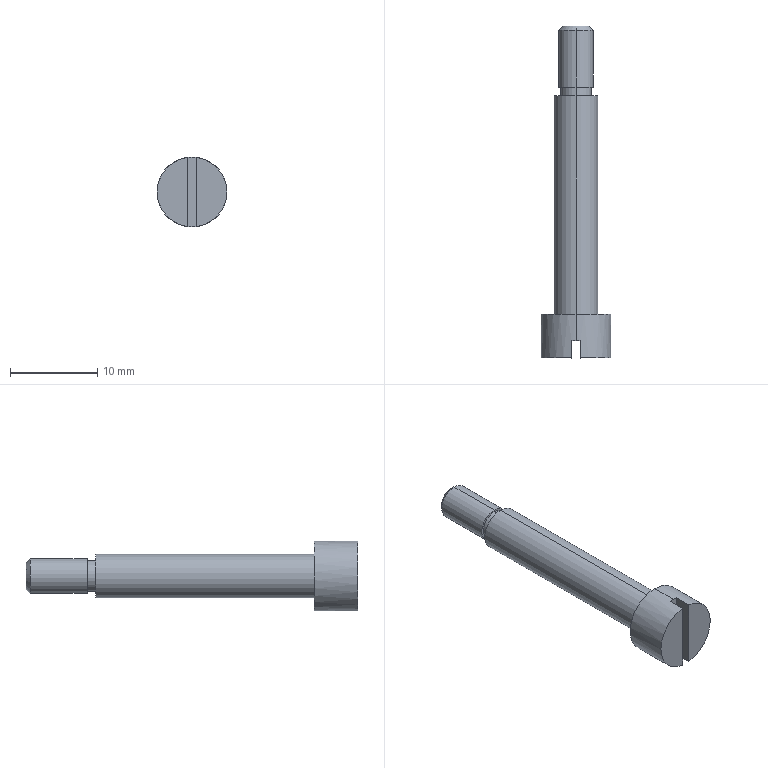Part | STEP file | 04-15 guide screw | 1 solid | 19 faces | box 8 x 38 x 8 mm | volume 822.389 mm3 | plane 9 | cylinder 8 | cone 2 | commonest cylinder face diameters 3.5 x2 4 x2 5 x2 8 x2
STEP:
#1=CARTESIAN_POINT('',(0.,7.,1.5));
#2=VERTEX_POINT('',#1);
#3=CARTESIAN_POINT('',(0.,7.,-1.5));
#4=VERTEX_POINT('',#3);
#5=CARTESIAN_POINT('',(0.,7.,0.));
#6=DIRECTION('',(0.,1.,0.));
#7=DIRECTION('',(0.,0.,1.));
#8=AXIS2_PLACEMENT_3D('',#5,#6,#7);
#9=CIRCLE('',#8,1.5);
#10=EDGE_CURVE('',#2,#4,#9,.T.);
#11=ORIENTED_EDGE('',*,*,#10,.F.);
#12=CARTESIAN_POINT('',(0.,6.5,2.));
#13=VERTEX_POINT('',#12);
#14=CARTESIAN_POINT('',(0.,7.,1.5));
#15=DIRECTION('',(0.,-0.7071,0.7071));
#16=VECTOR('',#15,1000.);
#17=LINE('',#14,#16);
#18=EDGE_CURVE('',#2,#13,#17,.T.);
#19=ORIENTED_EDGE('',*,*,#18,.T.);
#20=CARTESIAN_POINT('',(0.,6.5,-2.));
#21=VERTEX_POINT('',#20);
#22=CARTESIAN_POINT('',(0.,6.5,0.));
#23=DIRECTION('',(0.,-1.,0.));
#24=DIRECTION('',(0.,0.,1.));
#25=AXIS2_PLACEMENT_3D('',#22,#23,#24);
#26=CIRCLE('',#25,2.);
#27=EDGE_CURVE('',#21,#13,#26,.T.);
#28=ORIENTED_EDGE('',*,*,#27,.F.);
#29=CARTESIAN_POINT('',(0.,7.,-1.5));
#30=DIRECTION('',(0.,-0.7071,-0.7071));
#31=VECTOR('',#30,1000.);
#32=LINE('',#29,#31);
#33=EDGE_CURVE('',#4,#21,#32,.T.);
#34=ORIENTED_EDGE('',*,*,#33,.F.);
#35=EDGE_LOOP('',(#11,#19,#28,#34));
#36=FACE_OUTER_BOUND('',#35,.T.);
#37=CARTESIAN_POINT('',(0.,7.,0.));
#38=DIRECTION('',(0.,-1.,0.));
#39=DIRECTION('',(0.,0.,-1.));
#40=AXIS2_PLACEMENT_3D('',#37,#38,#39);
#41=CONICAL_SURFACE('',#40,1.5,0.7854);
#42=ADVANCED_FACE('',(#36),#41,.T.);
#43=CARTESIAN_POINT('',(0.,-29.,-4.));
#44=VERTEX_POINT('',#43);
#45=CARTESIAN_POINT('',(0.5,-29.,-3.969));
#46=VERTEX_POINT('',#45);
#47=CARTESIAN_POINT('',(0.,-29.,0.));
#48=DIRECTION('',(0.,-1.,0.));
#49=DIRECTION('',(0.,0.,-1.));
#50=AXIS2_PLACEMENT_3D('',#47,#48,#49);
#51=CIRCLE('',#50,4.);
#52=EDGE_CURVE('',#44,#46,#51,.T.);
#53=ORIENTED_EDGE('',*,*,#52,.F.);
#54=CARTESIAN_POINT('',(0.,-26.,-4.));
#55=VERTEX_POINT('',#54);
#56=CARTESIAN_POINT('',(0.,-31.,-4.));
#57=DIRECTION('',(0.,1.,0.));
#58=VECTOR('',#57,1000.);
#59=LINE('',#56,#58);
#60=EDGE_CURVE('',#44,#55,#59,.T.);
#61=ORIENTED_EDGE('',*,*,#60,.T.);
#62=CARTESIAN_POINT('',(0.,-26.,4.));
#63=VERTEX_POINT('',#62);
#64=CARTESIAN_POINT('',(0.,-26.,0.));
#65=DIRECTION('',(0.,-1.,0.));
#66=DIRECTION('',(0.,0.,-1.));
#67=AXIS2_PLACEMENT_3D('',#64,#65,#66);
#68=CIRCLE('',#67,4.);
#69=EDGE_CURVE('',#55,#63,#68,.T.);
#70=ORIENTED_EDGE('',*,*,#69,.T.);
#71=CARTESIAN_POINT('',(0.,-29.,4.));
#72=VERTEX_POINT('',#71);
#73=CARTESIAN_POINT('',(0.,-31.,4.));
#74=DIRECTION('',(0.,1.,0.));
#75=VECTOR('',#74,1000.);
#76=LINE('',#73,#75);
#77=EDGE_CURVE('',#72,#63,#76,.T.);
#78=ORIENTED_EDGE('',*,*,#77,.F.);
#79=CARTESIAN_POINT('',(0.5,-29.,3.969));
#80=VERTEX_POINT('',#79);
#81=CARTESIAN_POINT('',(0.,-29.,0.));
#82=DIRECTION('',(0.,-1.,0.));
#83=DIRECTION('',(0.,0.,-1.));
#84=AXIS2_PLACEMENT_3D('',#81,#82,#83);
#85=CIRCLE('',#84,4.);
#86=EDGE_CURVE('',#80,#72,#85,.T.);
#87=ORIENTED_EDGE('',*,*,#86,.F.);
#88=CARTESIAN_POINT('',(0.5,-31.,3.969));
#89=VERTEX_POINT('',#88);
#90=CARTESIAN_POINT('',(0.5,-31.,3.969));
#91=DIRECTION('',(0.,-1.,0.));
#92=VECTOR('',#91,1000.);
#93=LINE('',#90,#92);
#94=EDGE_CURVE('',#80,#89,#93,.T.);
#95=ORIENTED_EDGE('',*,*,#94,.T.);
#96=CARTESIAN_POINT('',(0.5,-31.,-3.969));
#97=VERTEX_POINT('',#96);
#98=CARTESIAN_POINT('',(0.,-31.,0.));
#99=DIRECTION('',(0.,-1.,0.));
#100=DIRECTION('',(0.,0.,-1.));
#101=AXIS2_PLACEMENT_3D('',#98,#99,#100);
#102=CIRCLE('',#101,4.);
#103=EDGE_CURVE('',#97,#89,#102,.T.);
#104=ORIENTED_EDGE('',*,*,#103,.F.);
#105=CARTESIAN_POINT('',(0.5,-31.,-3.969));
#106=DIRECTION('',(0.,1.,0.));
#107=VECTOR('',#106,1000.);
#108=LINE('',#105,#107);
#109=EDGE_CURVE('',#97,#46,#108,.T.);
#110=ORIENTED_EDGE('',*,*,#109,.T.);
#111=EDGE_LOOP('',(#53,#61,#70,#78,#87,#95,#104,#110));
#112=FACE_OUTER_BOUND('',#111,.T.);
#113=CARTESIAN_POINT('',(0.,-31.,0.));
#114=DIRECTION('',(0.,1.,0.));
#115=DIRECTION('',(0.,0.,1.));
#116=AXIS2_PLACEMENT_3D('',#113,#114,#115);
#117=CYLINDRICAL_SURFACE('',#116,4.);
#118=ADVANCED_FACE('',(#112),#117,.T.);
#119=CARTESIAN_POINT('',(0.,-26.,-2.5));
#120=VERTEX_POINT('',#119);
#121=CARTESIAN_POINT('',(0.,-26.,2.5));
#122=VERTEX_POINT('',#121);
#123=CARTESIAN_POINT('',(0.,-26.,0.));
#124=DIRECTION('',(0.,-1.,0.));
#125=DIRECTION('',(0.,0.,-1.));
#126=AXIS2_PLACEMENT_3D('',#123,#124,#125);
#127=CIRCLE('',#126,2.5);
#128=EDGE_CURVE('',#120,#122,#127,.T.);
#129=ORIENTED_EDGE('',*,*,#128,.F.);
#130=CARTESIAN_POINT('',(0.,-1.,-2.5));
#131=VERTEX_POINT('',#130);
#132=CARTESIAN_POINT('',(0.,-26.,-2.5));
#133=DIRECTION('',(0.,1.,0.));
#134=VECTOR('',#133,1000.);
#135=LINE('',#132,#134);
#136=EDGE_CURVE('',#120,#131,#135,.T.);
#137=ORIENTED_EDGE('',*,*,#136,.T.);
#138=CARTESIAN_POINT('',(0.,-1.,2.5));
#139=VERTEX_POINT('',#138);
#140=CARTESIAN_POINT('',(0.,-1.,0.));
#141=DIRECTION('',(0.,-1.,0.));
#142=DIRECTION('',(0.,0.,-1.));
#143=AXIS2_PLACEMENT_3D('',#140,#141,#142);
#144=CIRCLE('',#143,2.5);
#145=EDGE_CURVE('',#131,#139,#144,.T.);
#146=ORIENTED_EDGE('',*,*,#145,.T.);
#147=CARTESIAN_POINT('',(0.,-26.,2.5));
#148=DIRECTION('',(0.,1.,0.));
#149=VECTOR('',#148,1000.);
#150=LINE('',#147,#149);
#151=EDGE_CURVE('',#122,#139,#150,.T.);
#152=ORIENTED_EDGE('',*,*,#151,.F.);
#153=EDGE_LOOP('',(#129,#137,#146,#152));
#154=FACE_OUTER_BOUND('',#153,.T.);
#155=CARTESIAN_POINT('',(0.,-26.,0.));
#156=DIRECTION('',(0.,1.,0.));
#157=DIRECTION('',(0.,0.,1.));
#158=AXIS2_PLACEMENT_3D('',#155,#156,#157);
#159=CYLINDRICAL_SURFACE('',#158,2.5);
#160=ADVANCED_FACE('',(#154),#159,.T.);
#161=CARTESIAN_POINT('',(0.,-1.,-1.75));
#162=VERTEX_POINT('',#161);
#163=CARTESIAN_POINT('',(0.,-1.,1.75));
#164=VERTEX_POINT('',#163);
#165=CARTESIAN_POINT('',(0.,-1.,0.));
#166=DIRECTION('',(0.,-1.,0.));
#167=DIRECTION('',(0.,0.,-1.));
#168=AXIS2_PLACEMENT_3D('',#165,#166,#167);
#169=CIRCLE('',#168,1.75);
#170=EDGE_CURVE('',#162,#164,#169,.T.);
#171=ORIENTED_EDGE('',*,*,#170,.F.);
#172=CARTESIAN_POINT('',(0.,0.,-1.75));
#173=VERTEX_POINT('',#172);
#174=CARTESIAN_POINT('',(0.,-1.,-1.75));
#175=DIRECTION('',(0.,1.,0.));
#176=VECTOR('',#175,1000.);
#177=LINE('',#174,#176);
#178=EDGE_CURVE('',#162,#173,#177,.T.);
#179=ORIENTED_EDGE('',*,*,#178,.T.);
#180=CARTESIAN_POINT('',(0.,0.,1.75));
#181=VERTEX_POINT('',#180);
#182=CARTESIAN_POINT('',(0.,0.,0.));
#183=DIRECTION('',(0.,-1.,0.));
#184=DIRECTION('',(0.,0.,1.));
#185=AXIS2_PLACEMENT_3D('',#182,#183,#184);
#186=CIRCLE('',#185,1.75);
#187=EDGE_CURVE('',#173,#181,#186,.T.);
#188=ORIENTED_EDGE('',*,*,#187,.T.);
#189=CARTESIAN_POINT('',(0.,-1.,1.75));
#190=DIRECTION('',(0.,1.,0.));
#191=VECTOR('',#190,1000.);
#192=LINE('',#189,#191);
#193=EDGE_CURVE('',#164,#181,#192,.T.);
#194=ORIENTED_EDGE('',*,*,#193,.F.);
#195=EDGE_LOOP('',(#171,#179,#188,#194));
#196=FACE_OUTER_BOUND('',#195,.T.);
#197=CARTESIAN_POINT('',(0.,-1.,0.));
#198=DIRECTION('',(0.,1.,0.));
#199=DIRECTION('',(0.,0.,1.));
#200=AXIS2_PLACEMENT_3D('',#197,#198,#199);
#201=CYLINDRICAL_SURFACE('',#200,1.75);
#202=ADVANCED_FACE('',(#196),#201,.T.);
#203=ORIENTED_EDGE('',*,*,#27,.T.);
#204=CARTESIAN_POINT('',(0.,0.,2.));
#205=VERTEX_POINT('',#204);
#206=CARTESIAN_POINT('',(0.,7.,2.));
#207=DIRECTION('',(0.,-1.,0.));
#208=VECTOR('',#207,1000.);
#209=LINE('',#206,#208);
#210=EDGE_CURVE('',#13,#205,#209,.T.);
#211=ORIENTED_EDGE('',*,*,#210,.T.);
#212=CARTESIAN_POINT('',(0.,0.,-2.));
#213=VERTEX_POINT('',#212);
#214=CARTESIAN_POINT('',(0.,0.,0.));
#215=DIRECTION('',(0.,1.,0.));
#216=DIRECTION('',(0.,0.,1.));
#217=AXIS2_PLACEMENT_3D('',#214,#215,#216);
#218=CIRCLE('',#217,2.);
#219=EDGE_CURVE('',#205,#213,#218,.T.);
#220=ORIENTED_EDGE('',*,*,#219,.T.);
#221=CARTESIAN_POINT('',(0.,7.,-2.));
#222=DIRECTION('',(0.,-1.,0.));
#223=VECTOR('',#222,1000.);
#224=LINE('',#221,#223);
#225=EDGE_CURVE('',#21,#213,#224,.T.);
#226=ORIENTED_EDGE('',*,*,#225,.F.);
#227=EDGE_LOOP('',(#203,#211,#220,#226));
#228=FACE_OUTER_BOUND('',#227,.T.);
#229=CARTESIAN_POINT('',(0.,7.,0.));
#230=DIRECTION('',(0.,-1.,0.));
#231=DIRECTION('',(0.,0.,-1.));
#232=AXIS2_PLACEMENT_3D('',#229,#230,#231);
#233=CYLINDRICAL_SURFACE('',#232,2.);
#234=ADVANCED_FACE('',(#228),#233,.T.);
#235=CARTESIAN_POINT('',(0.5,-31.,0.));
#236=DIRECTION('',(0.,0.,1.));
#237=VECTOR('',#236,1000.);
#238=LINE('',#235,#237);
#239=EDGE_CURVE('',#97,#89,#238,.T.);
#240=ORIENTED_EDGE('',*,*,#239,.F.);
#241=ORIENTED_EDGE('',*,*,#103,.T.);
#242=EDGE_LOOP('',(#240,#241));
#243=FACE_OUTER_BOUND('',#242,.T.);
#244=CARTESIAN_POINT('',(0.,-31.,0.));
#245=DIRECTION('',(0.,-1.,0.));
#246=DIRECTION('',(0.,0.,-1.));
#247=AXIS2_PLACEMENT_3D('',#244,#245,#246);
#248=PLANE('',#247);
#249=ADVANCED_FACE('',(#243),#248,.T.);
#250=CARTESIAN_POINT('',(0.,0.,0.));
#251=DIRECTION('',(0.,1.,0.));
#252=DIRECTION('',(0.,0.,1.));
#253=AXIS2_PLACEMENT_3D('',#250,#251,#252);
#254=CIRCLE('',#253,2.);
#255=EDGE_CURVE('',#213,#205,#254,.T.);
#256=ORIENTED_EDGE('',*,*,#255,.F.);
#257=ORIENTED_EDGE('',*,*,#219,.F.);
#258=EDGE_LOOP('',(#256,#257));
#259=FACE_OUTER_BOUND('',#258,.T.);
#260=CARTESIAN_POINT('',(0.,0.,0.));
#261=DIRECTION('',(0.,-1.,0.));
#262=DIRECTION('',(0.,0.,1.));
#263=AXIS2_PLACEMENT_3D('',#260,#261,#262);
#264=CIRCLE('',#263,1.75);
#265=EDGE_CURVE('',#181,#173,#264,.T.);
#266=ORIENTED_EDGE('',*,*,#265,.F.);
#267=ORIENTED_EDGE('',*,*,#187,.F.);
#268=EDGE_LOOP('',(#266,#267));
#269=FACE_BOUND('',#268,.T.);
#270=CARTESIAN_POINT('',(0.,0.,0.));
#271=DIRECTION('',(0.,1.,0.));
#272=DIRECTION('',(0.,0.,1.));
#273=AXIS2_PLACEMENT_3D('',#270,#271,#272);
#274=PLANE('',#273);
#275=ADVANCED_FACE('',(#259,#269),#274,.F.);
#276=ORIENTED_EDGE('',*,*,#210,.F.);
#277=CARTESIAN_POINT('',(0.,6.5,0.));
#278=DIRECTION('',(0.,-1.,0.));
#279=DIRECTION('',(0.,0.,1.));
#280=AXIS2_PLACEMENT_3D('',#277,#278,#279);
#281=CIRCLE('',#280,2.);
#282=EDGE_CURVE('',#13,#21,#281,.T.);
#283=ORIENTED_EDGE('',*,*,#282,.T.);
#284=ORIENTED_EDGE('',*,*,#225,.T.);
#285=ORIENTED_EDGE('',*,*,#255,.T.);
#286=EDGE_LOOP('',(#276,#283,#284,#285));
#287=FACE_OUTER_BOUND('',#286,.T.);
#288=CARTESIAN_POINT('',(0.,7.,0.));
#289=DIRECTION('',(0.,-1.,0.));
#290=DIRECTION('',(0.,0.,-1.));
#291=AXIS2_PLACEMENT_3D('',#288,#289,#290);
#292=CYLINDRICAL_SURFACE('',#291,2.);
#293=ADVANCED_FACE('',(#287),#292,.T.);
#294=CARTESIAN_POINT('',(0.,7.,0.));
#295=DIRECTION('',(0.,1.,0.));
#296=DIRECTION('',(0.,0.,1.));
#297=AXIS2_PLACEMENT_3D('',#294,#295,#296);
#298=CIRCLE('',#297,1.5);
#299=EDGE_CURVE('',#4,#2,#298,.T.);
#300=ORIENTED_EDGE('',*,*,#299,.T.);
#301=ORIENTED_EDGE('',*,*,#10,.T.);
#302=EDGE_LOOP('',(#300,#301));
#303=FACE_OUTER_BOUND('',#302,.T.);
#304=CARTESIAN_POINT('',(0.,7.,0.));
#305=DIRECTION('',(0.,1.,0.));
#306=DIRECTION('',(0.,0.,1.));
#307=AXIS2_PLACEMENT_3D('',#304,#305,#306);
#308=PLANE('',#307);
#309=ADVANCED_FACE('',(#303),#308,.T.);
#310=ORIENTED_EDGE('',*,*,#178,.F.);
#311=CARTESIAN_POINT('',(0.,-1.,0.));
#312=DIRECTION('',(0.,-1.,0.));
#313=DIRECTION('',(0.,0.,-1.));
#314=AXIS2_PLACEMENT_3D('',#311,#312,#313);
#315=CIRCLE('',#314,1.75);
#316=EDGE_CURVE('',#164,#162,#315,.T.);
#317=ORIENTED_EDGE('',*,*,#316,.F.);
#318=ORIENTED_EDGE('',*,*,#193,.T.);
#319=ORIENTED_EDGE('',*,*,#265,.T.);
#320=EDGE_LOOP('',(#310,#317,#318,#319));
#321=FACE_OUTER_BOUND('',#320,.T.);
#322=CARTESIAN_POINT('',(0.,-1.,0.));
#323=DIRECTION('',(0.,1.,0.));
#324=DIRECTION('',(0.,0.,1.));
#325=AXIS2_PLACEMENT_3D('',#322,#323,#324);
#326=CYLINDRICAL_SURFACE('',#325,1.75);
#327=ADVANCED_FACE('',(#321),#326,.T.);
#328=CARTESIAN_POINT('',(0.,-1.,0.));
#329=DIRECTION('',(0.,-1.,0.));
#330=DIRECTION('',(0.,0.,-1.));
#331=AXIS2_PLACEMENT_3D('',#328,#329,#330);
#332=CIRCLE('',#331,2.5);
#333=EDGE_CURVE('',#139,#131,#332,.T.);
#334=ORIENTED_EDGE('',*,*,#333,.F.);
#335=ORIENTED_EDGE('',*,*,#145,.F.);
#336=EDGE_LOOP('',(#334,#335));
#337=FACE_OUTER_BOUND('',#336,.T.);
#338=ORIENTED_EDGE('',*,*,#316,.T.);
#339=ORIENTED_EDGE('',*,*,#170,.T.);
#340=EDGE_LOOP('',(#338,#339));
#341=FACE_BOUND('',#340,.T.);
#342=CARTESIAN_POINT('',(0.,-1.,0.));
#343=DIRECTION('',(0.,-1.,0.));
#344=DIRECTION('',(0.,0.,-1.));
#345=AXIS2_PLACEMENT_3D('',#342,#343,#344);
#346=PLANE('',#345);
#347=ADVANCED_FACE('',(#337,#341),#346,.F.);
#348=ORIENTED_EDGE('',*,*,#136,.F.);
#349=CARTESIAN_POINT('',(0.,-26.,0.));
#350=DIRECTION('',(0.,-1.,0.));
#351=DIRECTION('',(0.,0.,-1.));
#352=AXIS2_PLACEMENT_3D('',#349,#350,#351);
#353=CIRCLE('',#352,2.5);
#354=EDGE_CURVE('',#122,#120,#353,.T.);
#355=ORIENTED_EDGE('',*,*,#354,.F.);
#356=ORIENTED_EDGE('',*,*,#151,.T.);
#357=ORIENTED_EDGE('',*,*,#333,.T.);
#358=EDGE_LOOP('',(#348,#355,#356,#357));
#359=FACE_OUTER_BOUND('',#358,.T.);
#360=CARTESIAN_POINT('',(0.,-26.,0.));
#361=DIRECTION('',(0.,1.,0.));
#362=DIRECTION('',(0.,0.,1.));
#363=AXIS2_PLACEMENT_3D('',#360,#361,#362);
#364=CYLINDRICAL_SURFACE('',#363,2.5);
#365=ADVANCED_FACE('',(#359),#364,.T.);
#366=CARTESIAN_POINT('',(0.,-26.,0.));
#367=DIRECTION('',(0.,-1.,0.));
#368=DIRECTION('',(0.,0.,-1.));
#369=AXIS2_PLACEMENT_3D('',#366,#367,#368);
#370=CIRCLE('',#369,4.);
#371=EDGE_CURVE('',#63,#55,#370,.T.);
#372=ORIENTED_EDGE('',*,*,#371,.F.);
#373=ORIENTED_EDGE('',*,*,#69,.F.);
#374=EDGE_LOOP('',(#372,#373));
#375=FACE_OUTER_BOUND('',#374,.T.);
#376=ORIENTED_EDGE('',*,*,#354,.T.);
#377=ORIENTED_EDGE('',*,*,#128,.T.);
#378=EDGE_LOOP('',(#376,#377));
#379=FACE_BOUND('',#378,.T.);
#380=CARTESIAN_POINT('',(0.,-26.,0.));
#381=DIRECTION('',(0.,-1.,0.));
#382=DIRECTION('',(0.,0.,-1.));
#383=AXIS2_PLACEMENT_3D('',#380,#381,#382);
#384=PLANE('',#383);
#385=ADVANCED_FACE('',(#375,#379),#384,.F.);
#386=ORIENTED_EDGE('',*,*,#60,.F.);
#387=CARTESIAN_POINT('',(-0.5,-29.,-3.969));
#388=VERTEX_POINT('',#387);
#389=CARTESIAN_POINT('',(0.,-29.,0.));
#390=DIRECTION('',(0.,-1.,0.));
#391=DIRECTION('',(0.,0.,-1.));
#392=AXIS2_PLACEMENT_3D('',#389,#390,#391);
#393=CIRCLE('',#392,4.);
#394=EDGE_CURVE('',#388,#44,#393,.T.);
#395=ORIENTED_EDGE('',*,*,#394,.F.);
#396=CARTESIAN_POINT('',(-0.5,-31.,-3.969));
#397=VERTEX_POINT('',#396);
#398=CARTESIAN_POINT('',(-0.5,-31.,-3.969));
#399=DIRECTION('',(0.,-1.,0.));
#400=VECTOR('',#399,1000.);
#401=LINE('',#398,#400);
#402=EDGE_CURVE('',#388,#397,#401,.T.);
#403=ORIENTED_EDGE('',*,*,#402,.T.);
#404=CARTESIAN_POINT('',(-0.5,-31.,3.969));
#405=VERTEX_POINT('',#404);
#406=CARTESIAN_POINT('',(0.,-31.,0.));
#407=DIRECTION('',(0.,-1.,0.));
#408=DIRECTION('',(0.,0.,-1.));
#409=AXIS2_PLACEMENT_3D('',#406,#407,#408);
#410=CIRCLE('',#409,4.);
#411=EDGE_CURVE('',#405,#397,#410,.T.);
#412=ORIENTED_EDGE('',*,*,#411,.F.);
#413=CARTESIAN_POINT('',(-0.5,-29.,3.969));
#414=VERTEX_POINT('',#413);
#415=CARTESIAN_POINT('',(-0.5,-31.,3.969));
#416=DIRECTION('',(0.,1.,0.));
#417=VECTOR('',#416,1000.);
#418=LINE('',#415,#417);
#419=EDGE_CURVE('',#405,#414,#418,.T.);
#420=ORIENTED_EDGE('',*,*,#419,.T.);
#421=CARTESIAN_POINT('',(0.,-29.,0.));
#422=DIRECTION('',(0.,-1.,0.));
#423=DIRECTION('',(0.,0.,-1.));
#424=AXIS2_PLACEMENT_3D('',#421,#422,#423);
#425=CIRCLE('',#424,4.);
#426=EDGE_CURVE('',#72,#414,#425,.T.);
#427=ORIENTED_EDGE('',*,*,#426,.F.);
#428=ORIENTED_EDGE('',*,*,#77,.T.);
#429=ORIENTED_EDGE('',*,*,#371,.T.);
#430=EDGE_LOOP('',(#386,#395,#403,#412,#420,#427,#428,#429));
#431=FACE_OUTER_BOUND('',#430,.T.);
#432=CARTESIAN_POINT('',(0.,-31.,0.));
#433=DIRECTION('',(0.,1.,0.));
#434=DIRECTION('',(0.,0.,1.));
#435=AXIS2_PLACEMENT_3D('',#432,#433,#434);
#436=CYLINDRICAL_SURFACE('',#435,4.);
#437=ADVANCED_FACE('',(#431),#436,.T.);
#438=CARTESIAN_POINT('',(-0.5,-31.,0.));
#439=DIRECTION('',(0.,0.,-1.));
#440=VECTOR('',#439,1000.);
#441=LINE('',#438,#440);
#442=EDGE_CURVE('',#405,#397,#441,.T.);
#443=ORIENTED_EDGE('',*,*,#442,.F.);
#444=ORIENTED_EDGE('',*,*,#411,.T.);
#445=EDGE_LOOP('',(#443,#444));
#446=FACE_OUTER_BOUND('',#445,.T.);
#447=CARTESIAN_POINT('',(0.,-31.,0.));
#448=DIRECTION('',(0.,-1.,0.));
#449=DIRECTION('',(0.,0.,-1.));
#450=AXIS2_PLACEMENT_3D('',#447,#448,#449);
#451=PLANE('',#450);
#452=ADVANCED_FACE('',(#446),#451,.T.);
#453=ORIENTED_EDGE('',*,*,#18,.F.);
#454=ORIENTED_EDGE('',*,*,#299,.F.);
#455=ORIENTED_EDGE('',*,*,#33,.T.);
#456=ORIENTED_EDGE('',*,*,#282,.F.);
#457=EDGE_LOOP('',(#453,#454,#455,#456));
#458=FACE_OUTER_BOUND('',#457,.T.);
#459=CARTESIAN_POINT('',(0.,7.,0.));
#460=DIRECTION('',(0.,-1.,0.));
#461=DIRECTION('',(0.,0.,-1.));
#462=AXIS2_PLACEMENT_3D('',#459,#460,#461);
#463=CONICAL_SURFACE('',#462,1.5,0.7854);
#464=ADVANCED_FACE('',(#458),#463,.T.);
#465=ORIENTED_EDGE('',*,*,#86,.T.);
#466=ORIENTED_EDGE('',*,*,#426,.T.);
#467=CARTESIAN_POINT('',(-0.5,-29.,4.171));
#468=DIRECTION('',(0.,0.,-1.));
#469=VECTOR('',#468,1000.);
#470=LINE('',#467,#469);
#471=EDGE_CURVE('',#414,#388,#470,.T.);
#472=ORIENTED_EDGE('',*,*,#471,.T.);
#473=ORIENTED_EDGE('',*,*,#394,.T.);
#474=ORIENTED_EDGE('',*,*,#52,.T.);
#475=CARTESIAN_POINT('',(0.5,-29.,4.171));
#476=DIRECTION('',(0.,0.,1.));
#477=VECTOR('',#476,1000.);
#478=LINE('',#475,#477);
#479=EDGE_CURVE('',#46,#80,#478,.T.);
#480=ORIENTED_EDGE('',*,*,#479,.T.);
#481=EDGE_LOOP('',(#465,#466,#472,#473,#474,#480));
#482=FACE_OUTER_BOUND('',#481,.T.);
#483=CARTESIAN_POINT('',(0.5,-29.,-4.171));
#484=DIRECTION('',(0.,-1.,0.));
#485=DIRECTION('',(0.,0.,-1.));
#486=AXIS2_PLACEMENT_3D('',#483,#484,#485);
#487=PLANE('',#486);
#488=ADVANCED_FACE('',(#482),#487,.T.);
#489=ORIENTED_EDGE('',*,*,#239,.T.);
#490=ORIENTED_EDGE('',*,*,#94,.F.);
#491=ORIENTED_EDGE('',*,*,#479,.F.);
#492=ORIENTED_EDGE('',*,*,#109,.F.);
#493=EDGE_LOOP('',(#489,#490,#491,#492));
#494=FACE_OUTER_BOUND('',#493,.T.);
#495=CARTESIAN_POINT('',(0.5,-29.,4.171));
#496=DIRECTION('',(1.,0.,0.));
#497=DIRECTION('',(0.,0.,-1.));
#498=AXIS2_PLACEMENT_3D('',#495,#496,#497);
#499=PLANE('',#498);
#500=ADVANCED_FACE('',(#494),#499,.F.);
#501=ORIENTED_EDGE('',*,*,#442,.T.);
#502=ORIENTED_EDGE('',*,*,#402,.F.);
#503=ORIENTED_EDGE('',*,*,#471,.F.);
#504=ORIENTED_EDGE('',*,*,#419,.F.);
#505=EDGE_LOOP('',(#501,#502,#503,#504));
#506=FACE_OUTER_BOUND('',#505,.T.);
#507=CARTESIAN_POINT('',(-0.5,-29.,4.171));
#508=DIRECTION('',(-1.,0.,0.));
#509=DIRECTION('',(0.,0.,1.));
#510=AXIS2_PLACEMENT_3D('',#507,#508,#509);
#511=PLANE('',#510);
#512=ADVANCED_FACE('',(#506),#511,.F.);
#513=CLOSED_SHELL('',(#42,#118,#160,#202,#234,#249,#275,#293,#309,#327,#347,#365,#385,#437,#452,#464,#488,#500,#512));
#514=MANIFOLD_SOLID_BREP('',#513);
#515=CARTESIAN_POINT('',(0.,0.,0.));
#516=DIRECTION('',(0.,0.,1.));
#517=DIRECTION('',(1.,0.,0.));
#518=AXIS2_PLACEMENT_3D('',#515,#516,#517);
#519=(LENGTH_UNIT()NAMED_UNIT(*)SI_UNIT(.MILLI.,.METRE.));
#520=UNCERTAINTY_MEASURE_WITH_UNIT(LENGTH_MEASURE(0.00001),#519,'','');
#521=(NAMED_UNIT(*)PLANE_ANGLE_UNIT()SI_UNIT($,.RADIAN.));
#522=(NAMED_UNIT(*)SI_UNIT($,.STERADIAN.)SOLID_ANGLE_UNIT());
#523=(GEOMETRIC_REPRESENTATION_CONTEXT(3)GLOBAL_UNCERTAINTY_ASSIGNED_CONTEXT((#520))GLOBAL_UNIT_ASSIGNED_CONTEXT((#519,#521,#522))REPRESENTATION_CONTEXT('',''));
#524=ADVANCED_BREP_SHAPE_REPRESENTATION('',(#514,#518),#523);